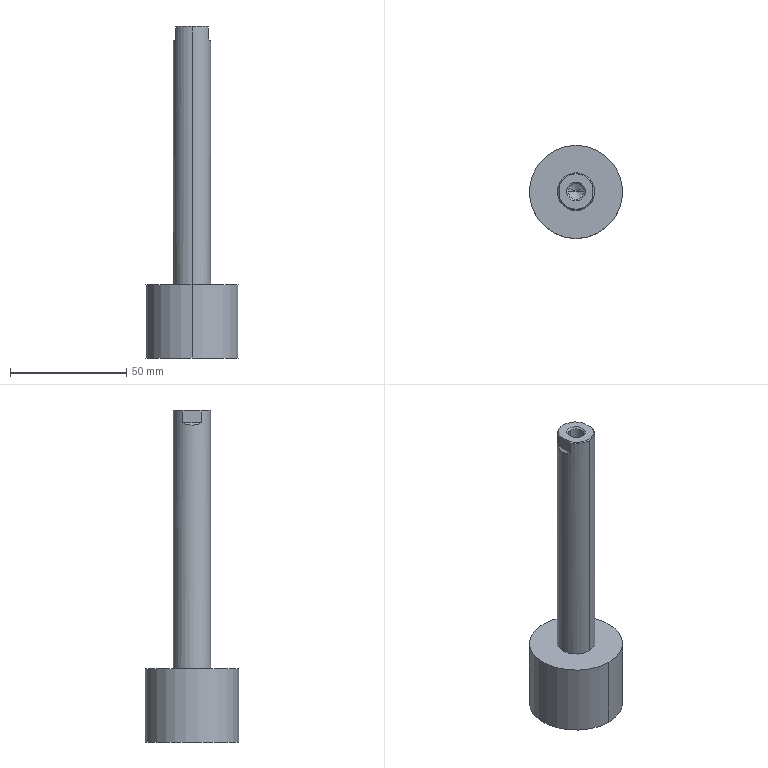Part | STEP file | HI_JSNR40X100_rod_default | 1 solid | 20 faces | box 40 x 40 x 142.5 mm | volume 61393 mm3 | cone 7 | plane 7 | cylinder 6 | commonest cylinder face diameters 6.647 x2 16 x2 40 x2